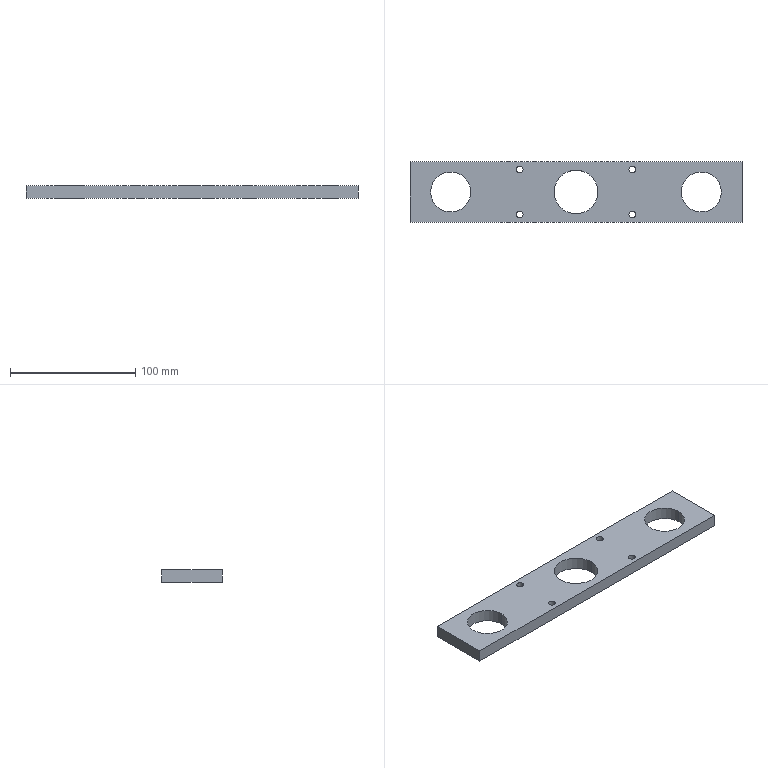Part | STEP file | B1-007 | 1 solid | 32 faces | box 265 x 48 x 10 mm | volume 99587 mm3 | cylinder 22 | plane 10 | commonest cylinder face diameters 5.5 x8 9 x8 32 x4 35 x2